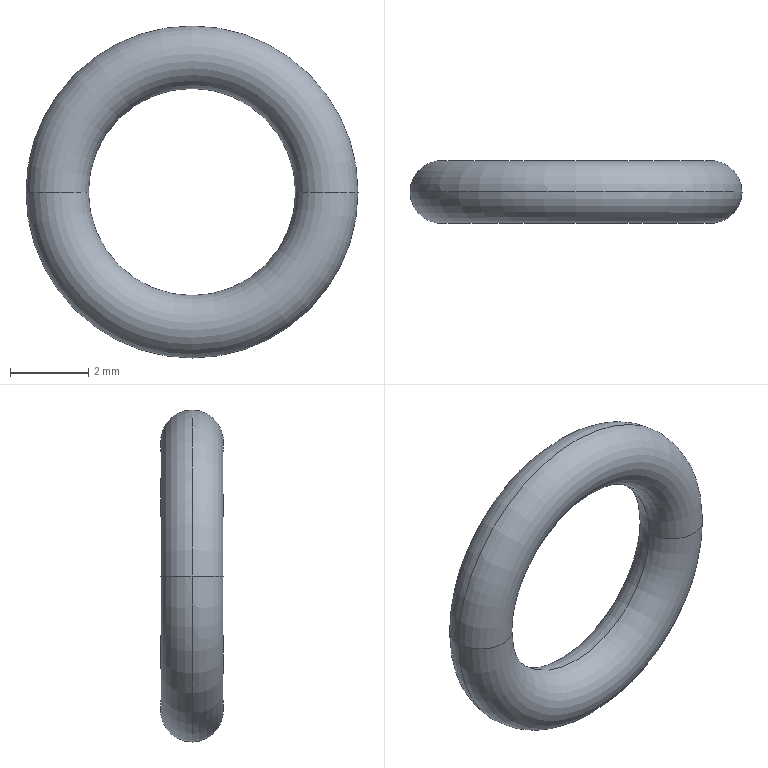Part | Creo | 1 solid | 4 faces | box 8.5 x 1.6 x 8.5 mm | volume 43.584 mm3 | torus 4
STEP:
#1=CARTESIAN_POINT('',(0.,0.,0.));
#2=DIRECTION('',(0.,0.,1.));
#3=DIRECTION('',(1.,0.,0.));
#4=AXIS2_PLACEMENT_3D('',#1,#2,#3);
#5=CARTESIAN_POINT('',(52.35,46.5,60.91));
#6=VERTEX_POINT('',#5);
#7=CARTESIAN_POINT('',(57.65,46.5,60.91));
#8=VERTEX_POINT('',#7);
#9=CARTESIAN_POINT('',(55.,46.5,60.91));
#10=DIRECTION('',(0.,1.,0.));
#11=DIRECTION('',(-1.,0.,0.));
#12=AXIS2_PLACEMENT_3D('',#9,#10,#11);
#13=CIRCLE('',#12,2.65);
#14=EDGE_CURVE('',#6,#8,#13,.T.);
#15=ORIENTED_EDGE('',*,*,#14,.F.);
#16=CARTESIAN_POINT('',(50.75,46.5,60.91));
#17=VERTEX_POINT('',#16);
#18=CARTESIAN_POINT('',(51.55,46.5,60.91));
#19=DIRECTION('',(0.,0.,-1.));
#20=DIRECTION('',(1.,0.,0.));
#21=AXIS2_PLACEMENT_3D('',#18,#19,#20);
#22=CIRCLE('',#21,0.8);
#23=EDGE_CURVE('',#6,#17,#22,.T.);
#24=ORIENTED_EDGE('',*,*,#23,.T.);
#25=CARTESIAN_POINT('',(59.25,46.5,60.91));
#26=VERTEX_POINT('',#25);
#27=CARTESIAN_POINT('',(55.,46.5,60.91));
#28=DIRECTION('',(0.,1.,0.));
#29=DIRECTION('',(-1.,0.,0.));
#30=AXIS2_PLACEMENT_3D('',#27,#28,#29);
#31=CIRCLE('',#30,4.25);
#32=EDGE_CURVE('',#17,#26,#31,.T.);
#33=ORIENTED_EDGE('',*,*,#32,.T.);
#34=CARTESIAN_POINT('',(58.45,46.5,60.91));
#35=DIRECTION('',(0.,0.,1.));
#36=DIRECTION('',(-1.,0.,0.));
#37=AXIS2_PLACEMENT_3D('',#34,#35,#36);
#38=CIRCLE('',#37,0.8);
#39=EDGE_CURVE('',#8,#26,#38,.T.);
#40=ORIENTED_EDGE('',*,*,#39,.F.);
#41=EDGE_LOOP('',(#15,#24,#33,#40));
#42=FACE_OUTER_BOUND('',#41,.F.);
#43=CARTESIAN_POINT('',(55.,46.5,60.91));
#44=DIRECTION('',(0.,1.,0.));
#45=DIRECTION('',(-1.,0.,0.));
#46=AXIS2_PLACEMENT_3D('',#43,#44,#45);
#47=TOROIDAL_SURFACE('',#46,3.45,0.8);
#48=ADVANCED_FACE('',(#42),#47,.T.);
#49=ORIENTED_EDGE('',*,*,#32,.F.);
#50=CARTESIAN_POINT('',(51.55,46.5,60.91));
#51=DIRECTION('',(0.,0.,-1.));
#52=DIRECTION('',(-1.,0.,0.));
#53=AXIS2_PLACEMENT_3D('',#50,#51,#52);
#54=CIRCLE('',#53,0.8);
#55=EDGE_CURVE('',#17,#6,#54,.T.);
#56=ORIENTED_EDGE('',*,*,#55,.T.);
#57=ORIENTED_EDGE('',*,*,#14,.T.);
#58=CARTESIAN_POINT('',(58.45,46.5,60.91));
#59=DIRECTION('',(0.,0.,1.));
#60=DIRECTION('',(1.,0.,0.));
#61=AXIS2_PLACEMENT_3D('',#58,#59,#60);
#62=CIRCLE('',#61,0.8);
#63=EDGE_CURVE('',#26,#8,#62,.T.);
#64=ORIENTED_EDGE('',*,*,#63,.F.);
#65=EDGE_LOOP('',(#49,#56,#57,#64));
#66=FACE_OUTER_BOUND('',#65,.F.);
#67=CARTESIAN_POINT('',(55.,46.5,60.91));
#68=DIRECTION('',(0.,1.,0.));
#69=DIRECTION('',(-1.,0.,0.));
#70=AXIS2_PLACEMENT_3D('',#67,#68,#69);
#71=TOROIDAL_SURFACE('',#70,3.45,0.8);
#72=ADVANCED_FACE('',(#66),#71,.T.);
#73=CARTESIAN_POINT('',(55.,46.5,60.91));
#74=DIRECTION('',(0.,1.,0.));
#75=DIRECTION('',(1.,0.,0.));
#76=AXIS2_PLACEMENT_3D('',#73,#74,#75);
#77=CIRCLE('',#76,4.25);
#78=EDGE_CURVE('',#26,#17,#77,.T.);
#79=ORIENTED_EDGE('',*,*,#78,.F.);
#80=ORIENTED_EDGE('',*,*,#63,.T.);
#81=CARTESIAN_POINT('',(55.,46.5,60.91));
#82=DIRECTION('',(0.,1.,0.));
#83=DIRECTION('',(1.,0.,0.));
#84=AXIS2_PLACEMENT_3D('',#81,#82,#83);
#85=CIRCLE('',#84,2.65);
#86=EDGE_CURVE('',#8,#6,#85,.T.);
#87=ORIENTED_EDGE('',*,*,#86,.T.);
#88=ORIENTED_EDGE('',*,*,#55,.F.);
#89=EDGE_LOOP('',(#79,#80,#87,#88));
#90=FACE_OUTER_BOUND('',#89,.F.);
#91=CARTESIAN_POINT('',(55.,46.5,60.91));
#92=DIRECTION('',(0.,1.,0.));
#93=DIRECTION('',(-1.,0.,0.));
#94=AXIS2_PLACEMENT_3D('',#91,#92,#93);
#95=TOROIDAL_SURFACE('',#94,3.45,0.8);
#96=ADVANCED_FACE('',(#90),#95,.T.);
#97=ORIENTED_EDGE('',*,*,#86,.F.);
#98=ORIENTED_EDGE('',*,*,#39,.T.);
#99=ORIENTED_EDGE('',*,*,#78,.T.);
#100=ORIENTED_EDGE('',*,*,#23,.F.);
#101=EDGE_LOOP('',(#97,#98,#99,#100));
#102=FACE_OUTER_BOUND('',#101,.F.);
#103=CARTESIAN_POINT('',(55.,46.5,60.91));
#104=DIRECTION('',(0.,1.,0.));
#105=DIRECTION('',(-1.,0.,0.));
#106=AXIS2_PLACEMENT_3D('',#103,#104,#105);
#107=TOROIDAL_SURFACE('',#106,3.45,0.8);
#108=ADVANCED_FACE('',(#102),#107,.T.);
#109=CLOSED_SHELL('',(#48,#72,#96,#108));
#110=MANIFOLD_SOLID_BREP('',#109);
#111=(LENGTH_UNIT()NAMED_UNIT(*)SI_UNIT(.MILLI.,.METRE.));
#112=UNCERTAINTY_MEASURE_WITH_UNIT(LENGTH_MEASURE(0.001213),#111,'','');
#113=(NAMED_UNIT(*)PLANE_ANGLE_UNIT()SI_UNIT($,.RADIAN.));
#114=PLANE_ANGLE_MEASURE_WITH_UNIT(PLANE_ANGLE_MEASURE(0.01745),#113);
#115=(CONVERSION_BASED_UNIT('DEGREE',#114)NAMED_UNIT(*)PLANE_ANGLE_UNIT());
#116=(NAMED_UNIT(*)SI_UNIT($,.STERADIAN.)SOLID_ANGLE_UNIT());
#117=(GEOMETRIC_REPRESENTATION_CONTEXT(3)GLOBAL_UNCERTAINTY_ASSIGNED_CONTEXT((#112))GLOBAL_UNIT_ASSIGNED_CONTEXT((#111,#115,#116))REPRESENTATION_CONTEXT('',''));
#118=ADVANCED_BREP_SHAPE_REPRESENTATION('',(#4,#110),#117);